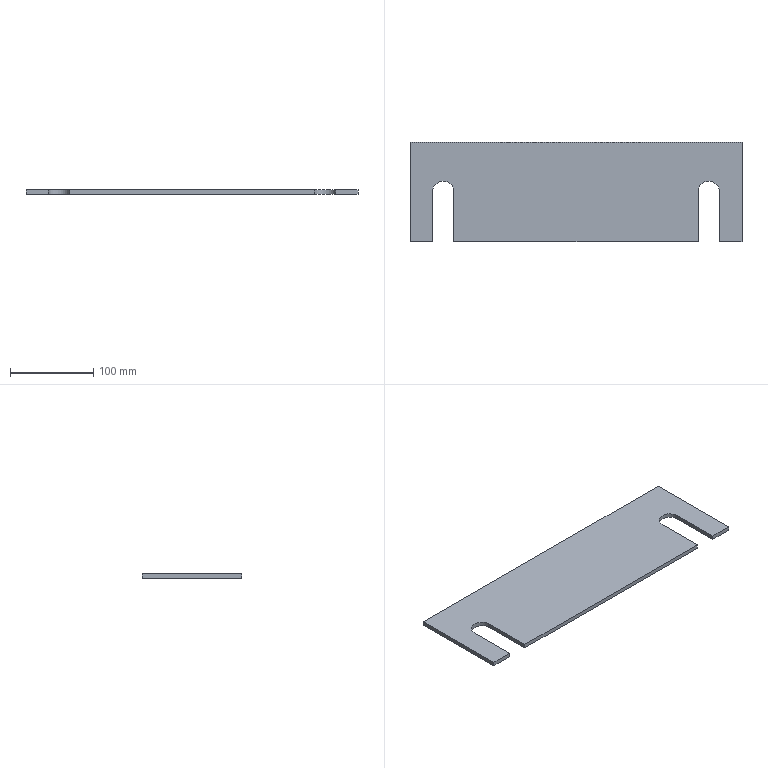Part | SolidWorks | features Extrusion 1, ICE 1 | 1 solid | 14 faces | box 400 x 120 x 5 mm | volume 221745 mm3 | plane 12 | cylinder 2 | commonest cylinder face diameters 26 x2
STEP:
#1=CARTESIAN_POINT('',(-147.,-60.,5.));
#2=VERTEX_POINT('',#1);
#3=CARTESIAN_POINT('',(147.,-60.,5.));
#4=VERTEX_POINT('',#3);
#5=CARTESIAN_POINT('',(-200.,-60.,5.));
#6=DIRECTION('',(1.,0.,0.));
#7=VECTOR('',#6,1000.);
#8=LINE('',#5,#7);
#9=EDGE_CURVE('',#2,#4,#8,.T.);
#10=ORIENTED_EDGE('',*,*,#9,.F.);
#11=CARTESIAN_POINT('',(-147.,-60.,0.));
#12=VERTEX_POINT('',#11);
#13=CARTESIAN_POINT('',(-147.,-60.,5.));
#14=DIRECTION('',(0.,0.,-1.));
#15=VECTOR('',#14,1000.);
#16=LINE('',#13,#15);
#17=EDGE_CURVE('',#2,#12,#16,.T.);
#18=ORIENTED_EDGE('',*,*,#17,.T.);
#19=CARTESIAN_POINT('',(147.,-60.,0.));
#20=VERTEX_POINT('',#19);
#21=CARTESIAN_POINT('',(-200.,-60.,0.));
#22=DIRECTION('',(1.,0.,0.));
#23=VECTOR('',#22,1000.);
#24=LINE('',#21,#23);
#25=EDGE_CURVE('',#12,#20,#24,.T.);
#26=ORIENTED_EDGE('',*,*,#25,.T.);
#27=CARTESIAN_POINT('',(147.,-60.,5.));
#28=DIRECTION('',(0.,0.,1.));
#29=VECTOR('',#28,1000.);
#30=LINE('',#27,#29);
#31=EDGE_CURVE('',#20,#4,#30,.T.);
#32=ORIENTED_EDGE('',*,*,#31,.T.);
#33=EDGE_LOOP('',(#10,#18,#26,#32));
#34=FACE_OUTER_BOUND('',#33,.T.);
#35=CARTESIAN_POINT('',(-200.,-60.,5.));
#36=DIRECTION('',(0.,1.,0.));
#37=DIRECTION('',(0.,0.,1.));
#38=AXIS2_PLACEMENT_3D('',#35,#36,#37);
#39=PLANE('',#38);
#40=ADVANCED_FACE('',(#34),#39,.F.);
#41=CARTESIAN_POINT('',(173.,-60.,5.));
#42=VERTEX_POINT('',#41);
#43=CARTESIAN_POINT('',(200.,-60.,5.));
#44=VERTEX_POINT('',#43);
#45=CARTESIAN_POINT('',(-200.,-60.,5.));
#46=DIRECTION('',(1.,0.,0.));
#47=VECTOR('',#46,1000.);
#48=LINE('',#45,#47);
#49=EDGE_CURVE('',#42,#44,#48,.T.);
#50=ORIENTED_EDGE('',*,*,#49,.F.);
#51=CARTESIAN_POINT('',(173.,-60.,0.));
#52=VERTEX_POINT('',#51);
#53=CARTESIAN_POINT('',(173.,-60.,5.));
#54=DIRECTION('',(0.,0.,-1.));
#55=VECTOR('',#54,1000.);
#56=LINE('',#53,#55);
#57=EDGE_CURVE('',#42,#52,#56,.T.);
#58=ORIENTED_EDGE('',*,*,#57,.T.);
#59=CARTESIAN_POINT('',(200.,-60.,0.));
#60=VERTEX_POINT('',#59);
#61=CARTESIAN_POINT('',(-200.,-60.,0.));
#62=DIRECTION('',(1.,0.,0.));
#63=VECTOR('',#62,1000.);
#64=LINE('',#61,#63);
#65=EDGE_CURVE('',#52,#60,#64,.T.);
#66=ORIENTED_EDGE('',*,*,#65,.T.);
#67=CARTESIAN_POINT('',(200.,-60.,5.));
#68=DIRECTION('',(0.,0.,-1.));
#69=VECTOR('',#68,1000.);
#70=LINE('',#67,#69);
#71=EDGE_CURVE('',#44,#60,#70,.T.);
#72=ORIENTED_EDGE('',*,*,#71,.F.);
#73=EDGE_LOOP('',(#50,#58,#66,#72));
#74=FACE_OUTER_BOUND('',#73,.T.);
#75=CARTESIAN_POINT('',(-200.,-60.,5.));
#76=DIRECTION('',(0.,1.,0.));
#77=DIRECTION('',(0.,0.,1.));
#78=AXIS2_PLACEMENT_3D('',#75,#76,#77);
#79=PLANE('',#78);
#80=ADVANCED_FACE('',(#74),#79,.F.);
#81=CARTESIAN_POINT('',(200.,60.,0.));
#82=VERTEX_POINT('',#81);
#83=CARTESIAN_POINT('',(200.,60.,0.));
#84=DIRECTION('',(0.,1.,0.));
#85=VECTOR('',#84,1000.);
#86=LINE('',#83,#85);
#87=EDGE_CURVE('',#60,#82,#86,.T.);
#88=ORIENTED_EDGE('',*,*,#87,.T.);
#89=CARTESIAN_POINT('',(200.,60.,5.));
#90=VERTEX_POINT('',#89);
#91=CARTESIAN_POINT('',(200.,60.,5.));
#92=DIRECTION('',(0.,0.,-1.));
#93=VECTOR('',#92,1000.);
#94=LINE('',#91,#93);
#95=EDGE_CURVE('',#90,#82,#94,.T.);
#96=ORIENTED_EDGE('',*,*,#95,.F.);
#97=CARTESIAN_POINT('',(200.,60.,5.));
#98=DIRECTION('',(0.,1.,0.));
#99=VECTOR('',#98,1000.);
#100=LINE('',#97,#99);
#101=EDGE_CURVE('',#44,#90,#100,.T.);
#102=ORIENTED_EDGE('',*,*,#101,.F.);
#103=ORIENTED_EDGE('',*,*,#71,.T.);
#104=EDGE_LOOP('',(#88,#96,#102,#103));
#105=FACE_OUTER_BOUND('',#104,.T.);
#106=CARTESIAN_POINT('',(200.,60.,5.));
#107=DIRECTION('',(-1.,0.,0.));
#108=DIRECTION('',(0.,-1.,0.));
#109=AXIS2_PLACEMENT_3D('',#106,#107,#108);
#110=PLANE('',#109);
#111=ADVANCED_FACE('',(#105),#110,.F.);
#112=CARTESIAN_POINT('',(-200.,60.,0.));
#113=VERTEX_POINT('',#112);
#114=CARTESIAN_POINT('',(-200.,60.,0.));
#115=DIRECTION('',(-1.,0.,0.));
#116=VECTOR('',#115,1000.);
#117=LINE('',#114,#116);
#118=EDGE_CURVE('',#82,#113,#117,.T.);
#119=ORIENTED_EDGE('',*,*,#118,.T.);
#120=CARTESIAN_POINT('',(-200.,60.,5.));
#121=VERTEX_POINT('',#120);
#122=CARTESIAN_POINT('',(-200.,60.,5.));
#123=DIRECTION('',(0.,0.,-1.));
#124=VECTOR('',#123,1000.);
#125=LINE('',#122,#124);
#126=EDGE_CURVE('',#121,#113,#125,.T.);
#127=ORIENTED_EDGE('',*,*,#126,.F.);
#128=CARTESIAN_POINT('',(-200.,60.,5.));
#129=DIRECTION('',(-1.,0.,0.));
#130=VECTOR('',#129,1000.);
#131=LINE('',#128,#130);
#132=EDGE_CURVE('',#90,#121,#131,.T.);
#133=ORIENTED_EDGE('',*,*,#132,.F.);
#134=ORIENTED_EDGE('',*,*,#95,.T.);
#135=EDGE_LOOP('',(#119,#127,#133,#134));
#136=FACE_OUTER_BOUND('',#135,.T.);
#137=CARTESIAN_POINT('',(-200.,60.,5.));
#138=DIRECTION('',(0.,-1.,0.));
#139=DIRECTION('',(0.,0.,-1.));
#140=AXIS2_PLACEMENT_3D('',#137,#138,#139);
#141=PLANE('',#140);
#142=ADVANCED_FACE('',(#136),#141,.F.);
#143=CARTESIAN_POINT('',(-200.,-60.,0.));
#144=VERTEX_POINT('',#143);
#145=CARTESIAN_POINT('',(-200.,60.,0.));
#146=DIRECTION('',(0.,-1.,0.));
#147=VECTOR('',#146,1000.);
#148=LINE('',#145,#147);
#149=EDGE_CURVE('',#113,#144,#148,.T.);
#150=ORIENTED_EDGE('',*,*,#149,.T.);
#151=CARTESIAN_POINT('',(-200.,-60.,5.));
#152=VERTEX_POINT('',#151);
#153=CARTESIAN_POINT('',(-200.,-60.,5.));
#154=DIRECTION('',(0.,0.,-1.));
#155=VECTOR('',#154,1000.);
#156=LINE('',#153,#155);
#157=EDGE_CURVE('',#152,#144,#156,.T.);
#158=ORIENTED_EDGE('',*,*,#157,.F.);
#159=CARTESIAN_POINT('',(-200.,60.,5.));
#160=DIRECTION('',(0.,-1.,0.));
#161=VECTOR('',#160,1000.);
#162=LINE('',#159,#161);
#163=EDGE_CURVE('',#121,#152,#162,.T.);
#164=ORIENTED_EDGE('',*,*,#163,.F.);
#165=ORIENTED_EDGE('',*,*,#126,.T.);
#166=EDGE_LOOP('',(#150,#158,#164,#165));
#167=FACE_OUTER_BOUND('',#166,.T.);
#168=CARTESIAN_POINT('',(-200.,60.,5.));
#169=DIRECTION('',(1.,0.,0.));
#170=DIRECTION('',(0.,1.,0.));
#171=AXIS2_PLACEMENT_3D('',#168,#169,#170);
#172=PLANE('',#171);
#173=ADVANCED_FACE('',(#167),#172,.F.);
#174=CARTESIAN_POINT('',(-173.,-60.,0.));
#175=VERTEX_POINT('',#174);
#176=CARTESIAN_POINT('',(-200.,-60.,0.));
#177=DIRECTION('',(1.,0.,0.));
#178=VECTOR('',#177,1000.);
#179=LINE('',#176,#178);
#180=EDGE_CURVE('',#144,#175,#179,.T.);
#181=ORIENTED_EDGE('',*,*,#180,.T.);
#182=CARTESIAN_POINT('',(-173.,-60.,5.));
#183=VERTEX_POINT('',#182);
#184=CARTESIAN_POINT('',(-173.,-60.,5.));
#185=DIRECTION('',(0.,0.,1.));
#186=VECTOR('',#185,1000.);
#187=LINE('',#184,#186);
#188=EDGE_CURVE('',#175,#183,#187,.T.);
#189=ORIENTED_EDGE('',*,*,#188,.T.);
#190=CARTESIAN_POINT('',(-200.,-60.,5.));
#191=DIRECTION('',(1.,0.,0.));
#192=VECTOR('',#191,1000.);
#193=LINE('',#190,#192);
#194=EDGE_CURVE('',#152,#183,#193,.T.);
#195=ORIENTED_EDGE('',*,*,#194,.F.);
#196=ORIENTED_EDGE('',*,*,#157,.T.);
#197=EDGE_LOOP('',(#181,#189,#195,#196));
#198=FACE_OUTER_BOUND('',#197,.T.);
#199=CARTESIAN_POINT('',(-200.,-60.,5.));
#200=DIRECTION('',(0.,1.,0.));
#201=DIRECTION('',(0.,0.,1.));
#202=AXIS2_PLACEMENT_3D('',#199,#200,#201);
#203=PLANE('',#202);
#204=ADVANCED_FACE('',(#198),#203,.F.);
#205=CARTESIAN_POINT('',(-147.,0.,5.));
#206=VERTEX_POINT('',#205);
#207=CARTESIAN_POINT('',(-147.,0.,5.));
#208=DIRECTION('',(0.,1.,0.));
#209=VECTOR('',#208,1000.);
#210=LINE('',#207,#209);
#211=EDGE_CURVE('',#2,#206,#210,.T.);
#212=ORIENTED_EDGE('',*,*,#211,.F.);
#213=ORIENTED_EDGE('',*,*,#9,.T.);
#214=CARTESIAN_POINT('',(147.,0.,5.));
#215=VERTEX_POINT('',#214);
#216=CARTESIAN_POINT('',(147.,0.,5.));
#217=DIRECTION('',(0.,-1.,0.));
#218=VECTOR('',#217,1000.);
#219=LINE('',#216,#218);
#220=EDGE_CURVE('',#215,#4,#219,.T.);
#221=ORIENTED_EDGE('',*,*,#220,.F.);
#222=CARTESIAN_POINT('',(173.,0.,5.));
#223=VERTEX_POINT('',#222);
#224=CARTESIAN_POINT('',(160.,0.,5.));
#225=DIRECTION('',(0.,0.,1.));
#226=DIRECTION('',(-1.,0.,0.));
#227=AXIS2_PLACEMENT_3D('',#224,#225,#226);
#228=CIRCLE('',#227,13.);
#229=EDGE_CURVE('',#223,#215,#228,.T.);
#230=ORIENTED_EDGE('',*,*,#229,.F.);
#231=CARTESIAN_POINT('',(173.,0.,5.));
#232=DIRECTION('',(0.,1.,0.));
#233=VECTOR('',#232,1000.);
#234=LINE('',#231,#233);
#235=EDGE_CURVE('',#42,#223,#234,.T.);
#236=ORIENTED_EDGE('',*,*,#235,.F.);
#237=ORIENTED_EDGE('',*,*,#49,.T.);
#238=ORIENTED_EDGE('',*,*,#101,.T.);
#239=ORIENTED_EDGE('',*,*,#132,.T.);
#240=ORIENTED_EDGE('',*,*,#163,.T.);
#241=ORIENTED_EDGE('',*,*,#194,.T.);
#242=CARTESIAN_POINT('',(-173.,0.,5.));
#243=VERTEX_POINT('',#242);
#244=CARTESIAN_POINT('',(-173.,0.,5.));
#245=DIRECTION('',(0.,-1.,0.));
#246=VECTOR('',#245,1000.);
#247=LINE('',#244,#246);
#248=EDGE_CURVE('',#243,#183,#247,.T.);
#249=ORIENTED_EDGE('',*,*,#248,.F.);
#250=CARTESIAN_POINT('',(-160.,0.,5.));
#251=DIRECTION('',(0.,0.,1.));
#252=DIRECTION('',(1.,0.,0.));
#253=AXIS2_PLACEMENT_3D('',#250,#251,#252);
#254=CIRCLE('',#253,13.);
#255=EDGE_CURVE('',#206,#243,#254,.T.);
#256=ORIENTED_EDGE('',*,*,#255,.F.);
#257=EDGE_LOOP('',(#212,#213,#221,#230,#236,#237,#238,#239,#240,#241,#249,#256));
#258=FACE_OUTER_BOUND('',#257,.T.);
#259=CARTESIAN_POINT('',(0.,0.,5.));
#260=DIRECTION('',(0.,0.,1.));
#261=DIRECTION('',(1.,0.,0.));
#262=AXIS2_PLACEMENT_3D('',#259,#260,#261);
#263=PLANE('',#262);
#264=ADVANCED_FACE('',(#258),#263,.T.);
#265=ORIENTED_EDGE('',*,*,#25,.F.);
#266=CARTESIAN_POINT('',(-147.,0.,0.));
#267=VERTEX_POINT('',#266);
#268=CARTESIAN_POINT('',(-147.,0.,0.));
#269=DIRECTION('',(0.,1.,0.));
#270=VECTOR('',#269,1000.);
#271=LINE('',#268,#270);
#272=EDGE_CURVE('',#12,#267,#271,.T.);
#273=ORIENTED_EDGE('',*,*,#272,.T.);
#274=CARTESIAN_POINT('',(-173.,0.,0.));
#275=VERTEX_POINT('',#274);
#276=CARTESIAN_POINT('',(-160.,0.,0.));
#277=DIRECTION('',(0.,0.,1.));
#278=DIRECTION('',(1.,0.,0.));
#279=AXIS2_PLACEMENT_3D('',#276,#277,#278);
#280=CIRCLE('',#279,13.);
#281=EDGE_CURVE('',#267,#275,#280,.T.);
#282=ORIENTED_EDGE('',*,*,#281,.T.);
#283=CARTESIAN_POINT('',(-173.,0.,0.));
#284=DIRECTION('',(0.,-1.,0.));
#285=VECTOR('',#284,1000.);
#286=LINE('',#283,#285);
#287=EDGE_CURVE('',#275,#175,#286,.T.);
#288=ORIENTED_EDGE('',*,*,#287,.T.);
#289=ORIENTED_EDGE('',*,*,#180,.F.);
#290=ORIENTED_EDGE('',*,*,#149,.F.);
#291=ORIENTED_EDGE('',*,*,#118,.F.);
#292=ORIENTED_EDGE('',*,*,#87,.F.);
#293=ORIENTED_EDGE('',*,*,#65,.F.);
#294=CARTESIAN_POINT('',(173.,0.,0.));
#295=VERTEX_POINT('',#294);
#296=CARTESIAN_POINT('',(173.,0.,0.));
#297=DIRECTION('',(0.,1.,0.));
#298=VECTOR('',#297,1000.);
#299=LINE('',#296,#298);
#300=EDGE_CURVE('',#52,#295,#299,.T.);
#301=ORIENTED_EDGE('',*,*,#300,.T.);
#302=CARTESIAN_POINT('',(147.,0.,0.));
#303=VERTEX_POINT('',#302);
#304=CARTESIAN_POINT('',(160.,0.,0.));
#305=DIRECTION('',(0.,0.,1.));
#306=DIRECTION('',(-1.,0.,0.));
#307=AXIS2_PLACEMENT_3D('',#304,#305,#306);
#308=CIRCLE('',#307,13.);
#309=EDGE_CURVE('',#295,#303,#308,.T.);
#310=ORIENTED_EDGE('',*,*,#309,.T.);
#311=CARTESIAN_POINT('',(147.,0.,0.));
#312=DIRECTION('',(0.,-1.,0.));
#313=VECTOR('',#312,1000.);
#314=LINE('',#311,#313);
#315=EDGE_CURVE('',#303,#20,#314,.T.);
#316=ORIENTED_EDGE('',*,*,#315,.T.);
#317=EDGE_LOOP('',(#265,#273,#282,#288,#289,#290,#291,#292,#293,#301,#310,#316));
#318=FACE_OUTER_BOUND('',#317,.T.);
#319=CARTESIAN_POINT('',(0.,0.,0.));
#320=DIRECTION('',(0.,0.,1.));
#321=DIRECTION('',(1.,0.,0.));
#322=AXIS2_PLACEMENT_3D('',#319,#320,#321);
#323=PLANE('',#322);
#324=ADVANCED_FACE('',(#318),#323,.F.);
#325=ORIENTED_EDGE('',*,*,#235,.T.);
#326=CARTESIAN_POINT('',(173.,0.,0.));
#327=DIRECTION('',(0.,0.,1.));
#328=VECTOR('',#327,1000.);
#329=LINE('',#326,#328);
#330=EDGE_CURVE('',#295,#223,#329,.T.);
#331=ORIENTED_EDGE('',*,*,#330,.F.);
#332=ORIENTED_EDGE('',*,*,#300,.F.);
#333=ORIENTED_EDGE('',*,*,#57,.F.);
#334=EDGE_LOOP('',(#325,#331,#332,#333));
#335=FACE_OUTER_BOUND('',#334,.T.);
#336=CARTESIAN_POINT('',(173.,0.,0.));
#337=DIRECTION('',(1.,0.,0.));
#338=DIRECTION('',(0.,1.,0.));
#339=AXIS2_PLACEMENT_3D('',#336,#337,#338);
#340=PLANE('',#339);
#341=ADVANCED_FACE('',(#335),#340,.F.);
#342=ORIENTED_EDGE('',*,*,#315,.F.);
#343=CARTESIAN_POINT('',(147.,0.,0.));
#344=DIRECTION('',(0.,0.,1.));
#345=VECTOR('',#344,1000.);
#346=LINE('',#343,#345);
#347=EDGE_CURVE('',#303,#215,#346,.T.);
#348=ORIENTED_EDGE('',*,*,#347,.T.);
#349=ORIENTED_EDGE('',*,*,#220,.T.);
#350=ORIENTED_EDGE('',*,*,#31,.F.);
#351=EDGE_LOOP('',(#342,#348,#349,#350));
#352=FACE_OUTER_BOUND('',#351,.T.);
#353=CARTESIAN_POINT('',(147.,0.,0.));
#354=DIRECTION('',(-1.,0.,0.));
#355=DIRECTION('',(0.,0.,1.));
#356=AXIS2_PLACEMENT_3D('',#353,#354,#355);
#357=PLANE('',#356);
#358=ADVANCED_FACE('',(#352),#357,.F.);
#359=ORIENTED_EDGE('',*,*,#229,.T.);
#360=ORIENTED_EDGE('',*,*,#347,.F.);
#361=ORIENTED_EDGE('',*,*,#309,.F.);
#362=ORIENTED_EDGE('',*,*,#330,.T.);
#363=EDGE_LOOP('',(#359,#360,#361,#362));
#364=FACE_OUTER_BOUND('',#363,.T.);
#365=CARTESIAN_POINT('',(160.,0.,0.));
#366=DIRECTION('',(0.,0.,1.));
#367=DIRECTION('',(1.,0.,0.));
#368=AXIS2_PLACEMENT_3D('',#365,#366,#367);
#369=CYLINDRICAL_SURFACE('',#368,13.);
#370=ADVANCED_FACE('',(#364),#369,.F.);
#371=ORIENTED_EDGE('',*,*,#211,.T.);
#372=CARTESIAN_POINT('',(-147.,0.,0.));
#373=DIRECTION('',(0.,0.,1.));
#374=VECTOR('',#373,1000.);
#375=LINE('',#372,#374);
#376=EDGE_CURVE('',#267,#206,#375,.T.);
#377=ORIENTED_EDGE('',*,*,#376,.F.);
#378=ORIENTED_EDGE('',*,*,#272,.F.);
#379=ORIENTED_EDGE('',*,*,#17,.F.);
#380=EDGE_LOOP('',(#371,#377,#378,#379));
#381=FACE_OUTER_BOUND('',#380,.T.);
#382=CARTESIAN_POINT('',(-147.,0.,0.));
#383=DIRECTION('',(1.,0.,0.));
#384=DIRECTION('',(0.,0.,-1.));
#385=AXIS2_PLACEMENT_3D('',#382,#383,#384);
#386=PLANE('',#385);
#387=ADVANCED_FACE('',(#381),#386,.F.);
#388=ORIENTED_EDGE('',*,*,#287,.F.);
#389=CARTESIAN_POINT('',(-173.,0.,0.));
#390=DIRECTION('',(0.,0.,1.));
#391=VECTOR('',#390,1000.);
#392=LINE('',#389,#391);
#393=EDGE_CURVE('',#275,#243,#392,.T.);
#394=ORIENTED_EDGE('',*,*,#393,.T.);
#395=ORIENTED_EDGE('',*,*,#248,.T.);
#396=ORIENTED_EDGE('',*,*,#188,.F.);
#397=EDGE_LOOP('',(#388,#394,#395,#396));
#398=FACE_OUTER_BOUND('',#397,.T.);
#399=CARTESIAN_POINT('',(-173.,0.,0.));
#400=DIRECTION('',(-1.,0.,0.));
#401=DIRECTION('',(0.,-1.,0.));
#402=AXIS2_PLACEMENT_3D('',#399,#400,#401);
#403=PLANE('',#402);
#404=ADVANCED_FACE('',(#398),#403,.F.);
#405=ORIENTED_EDGE('',*,*,#255,.T.);
#406=ORIENTED_EDGE('',*,*,#393,.F.);
#407=ORIENTED_EDGE('',*,*,#281,.F.);
#408=ORIENTED_EDGE('',*,*,#376,.T.);
#409=EDGE_LOOP('',(#405,#406,#407,#408));
#410=FACE_OUTER_BOUND('',#409,.T.);
#411=CARTESIAN_POINT('',(-160.,0.,0.));
#412=DIRECTION('',(0.,0.,1.));
#413=DIRECTION('',(1.,0.,0.));
#414=AXIS2_PLACEMENT_3D('',#411,#412,#413);
#415=CYLINDRICAL_SURFACE('',#414,13.);
#416=ADVANCED_FACE('',(#410),#415,.F.);
#417=CLOSED_SHELL('',(#40,#80,#111,#142,#173,#204,#264,#324,#341,#358,#370,#387,#404,#416));
#418=MANIFOLD_SOLID_BREP('',#417);
#419=CARTESIAN_POINT('',(0.,0.,0.));
#420=DIRECTION('',(0.,0.,1.));
#421=DIRECTION('',(1.,0.,0.));
#422=AXIS2_PLACEMENT_3D('',#419,#420,#421);
#423=(LENGTH_UNIT()NAMED_UNIT(*)SI_UNIT(.MILLI.,.METRE.));
#424=UNCERTAINTY_MEASURE_WITH_UNIT(LENGTH_MEASURE(0.00001),#423,'','');
#425=(NAMED_UNIT(*)PLANE_ANGLE_UNIT()SI_UNIT($,.RADIAN.));
#426=(NAMED_UNIT(*)SI_UNIT($,.STERADIAN.)SOLID_ANGLE_UNIT());
#427=(GEOMETRIC_REPRESENTATION_CONTEXT(3)GLOBAL_UNCERTAINTY_ASSIGNED_CONTEXT((#424))GLOBAL_UNIT_ASSIGNED_CONTEXT((#423,#425,#426))REPRESENTATION_CONTEXT('',''));
#428=ADVANCED_BREP_SHAPE_REPRESENTATION('',(#418,#422),#427);